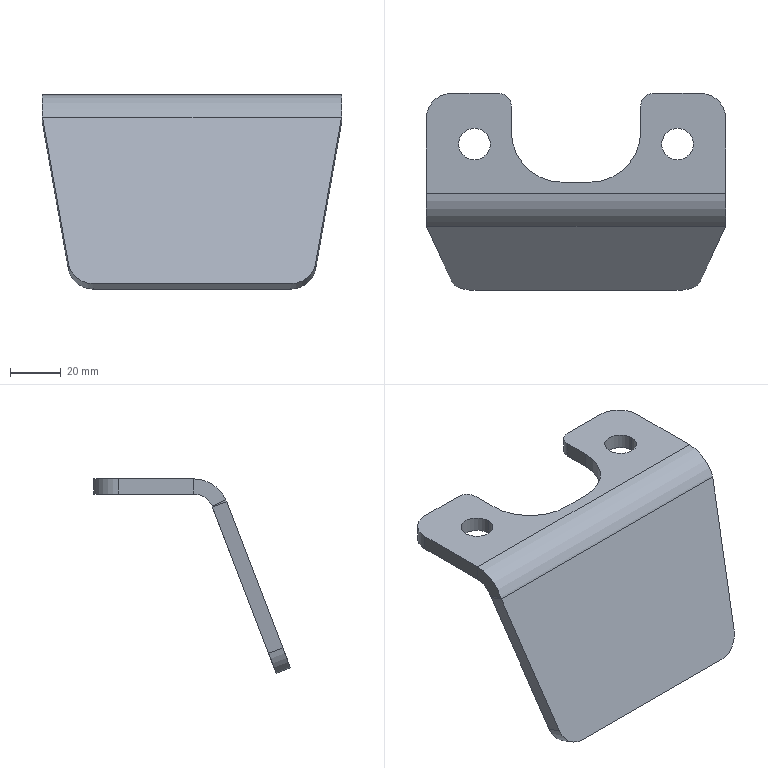Part | SolidWorks | features FlatPattern 1, SM3dBend 1, SMBaseFlange 1, SheetMetal 1, UnFold 1 | 1 solid | 32 faces | box 118 x 77.569 x 76.575 mm | volume 70276 mm3 | plane 16 | cylinder 14 | spline 2 | commonest cylinder face diameters 12.5 x4 20 x4 10 x2 40 x2 16 x1 28 x1
STEP:
#1=CARTESIAN_POINT('',(12.75,-20.,6.));
#2=VERTEX_POINT('',#1);
#3=CARTESIAN_POINT('',(25.25,-20.,6.));
#4=VERTEX_POINT('',#3);
#5=CARTESIAN_POINT('',(19.,-20.,6.));
#6=DIRECTION('',(0.,0.,1.));
#7=DIRECTION('',(1.,0.,0.));
#8=AXIS2_PLACEMENT_3D('',#5,#6,#7);
#9=CIRCLE('',#8,6.25);
#10=EDGE_CURVE('',#2,#4,#9,.T.);
#11=ORIENTED_EDGE('',*,*,#10,.T.);
#12=CARTESIAN_POINT('',(25.25,-20.,0.));
#13=VERTEX_POINT('',#12);
#14=CARTESIAN_POINT('',(25.25,-20.,6.));
#15=DIRECTION('',(0.,0.,-1.));
#16=VECTOR('',#15,1000.);
#17=LINE('',#14,#16);
#18=EDGE_CURVE('',#4,#13,#17,.T.);
#19=ORIENTED_EDGE('',*,*,#18,.T.);
#20=CARTESIAN_POINT('',(12.75,-20.,0.));
#21=VERTEX_POINT('',#20);
#22=CARTESIAN_POINT('',(19.,-20.,0.));
#23=DIRECTION('',(0.,0.,1.));
#24=DIRECTION('',(1.,0.,0.));
#25=AXIS2_PLACEMENT_3D('',#22,#23,#24);
#26=CIRCLE('',#25,6.25);
#27=EDGE_CURVE('',#21,#13,#26,.T.);
#28=ORIENTED_EDGE('',*,*,#27,.F.);
#29=CARTESIAN_POINT('',(12.75,-20.,6.));
#30=DIRECTION('',(0.,0.,-1.));
#31=VECTOR('',#30,1000.);
#32=LINE('',#29,#31);
#33=EDGE_CURVE('',#2,#21,#32,.T.);
#34=ORIENTED_EDGE('',*,*,#33,.F.);
#35=EDGE_LOOP('',(#11,#19,#28,#34));
#36=FACE_OUTER_BOUND('',#35,.T.);
#37=CARTESIAN_POINT('',(19.,-20.,6.));
#38=DIRECTION('',(0.,0.,-1.));
#39=DIRECTION('',(-1.,0.,0.));
#40=AXIS2_PLACEMENT_3D('',#37,#38,#39);
#41=CYLINDRICAL_SURFACE('',#40,6.25);
#42=ADVANCED_FACE('',(#36),#41,.F.);
#43=CARTESIAN_POINT('',(92.75,-20.,6.));
#44=VERTEX_POINT('',#43);
#45=CARTESIAN_POINT('',(105.25,-20.,6.));
#46=VERTEX_POINT('',#45);
#47=CARTESIAN_POINT('',(99.,-20.,6.));
#48=DIRECTION('',(0.,0.,1.));
#49=DIRECTION('',(1.,0.,0.));
#50=AXIS2_PLACEMENT_3D('',#47,#48,#49);
#51=CIRCLE('',#50,6.25);
#52=EDGE_CURVE('',#44,#46,#51,.T.);
#53=ORIENTED_EDGE('',*,*,#52,.T.);
#54=CARTESIAN_POINT('',(105.25,-20.,0.));
#55=VERTEX_POINT('',#54);
#56=CARTESIAN_POINT('',(105.25,-20.,6.));
#57=DIRECTION('',(0.,0.,-1.));
#58=VECTOR('',#57,1000.);
#59=LINE('',#56,#58);
#60=EDGE_CURVE('',#46,#55,#59,.T.);
#61=ORIENTED_EDGE('',*,*,#60,.T.);
#62=CARTESIAN_POINT('',(92.75,-20.,0.));
#63=VERTEX_POINT('',#62);
#64=CARTESIAN_POINT('',(99.,-20.,0.));
#65=DIRECTION('',(0.,0.,1.));
#66=DIRECTION('',(1.,0.,0.));
#67=AXIS2_PLACEMENT_3D('',#64,#65,#66);
#68=CIRCLE('',#67,6.25);
#69=EDGE_CURVE('',#63,#55,#68,.T.);
#70=ORIENTED_EDGE('',*,*,#69,.F.);
#71=CARTESIAN_POINT('',(92.75,-20.,6.));
#72=DIRECTION('',(0.,0.,-1.));
#73=VECTOR('',#72,1000.);
#74=LINE('',#71,#73);
#75=EDGE_CURVE('',#44,#63,#74,.T.);
#76=ORIENTED_EDGE('',*,*,#75,.F.);
#77=EDGE_LOOP('',(#53,#61,#70,#76));
#78=FACE_OUTER_BOUND('',#77,.T.);
#79=CARTESIAN_POINT('',(99.,-20.,6.));
#80=DIRECTION('',(0.,0.,-1.));
#81=DIRECTION('',(-1.,0.,0.));
#82=AXIS2_PLACEMENT_3D('',#79,#80,#81);
#83=CYLINDRICAL_SURFACE('',#82,6.25);
#84=ADVANCED_FACE('',(#78),#83,.F.);
#85=CARTESIAN_POINT('',(107.685,-74.57,-60.613));
#86=VERTEX_POINT('',#85);
#87=CARTESIAN_POINT('',(117.9,-52.448,-2.983));
#88=VERTEX_POINT('',#87);
#89=CARTESIAN_POINT('',(107.685,-74.57,-60.613));
#90=DIRECTION('',(0.1633,0.3536,0.9211));
#91=VECTOR('',#90,1000.);
#92=LINE('',#89,#91);
#93=EDGE_CURVE('',#86,#88,#92,.T.);
#94=ORIENTED_EDGE('',*,*,#93,.T.);
#95=CARTESIAN_POINT('',(0.09971,-52.448,-2.983));
#96=VERTEX_POINT('',#95);
#97=CARTESIAN_POINT('',(20.181,-52.448,-2.983));
#98=DIRECTION('',(-1.,0.,0.));
#99=VECTOR('',#98,1000.);
#100=LINE('',#97,#99);
#101=EDGE_CURVE('',#88,#96,#100,.T.);
#102=ORIENTED_EDGE('',*,*,#101,.T.);
#103=CARTESIAN_POINT('',(10.315,-74.57,-60.613));
#104=VERTEX_POINT('',#103);
#105=CARTESIAN_POINT('',(0.,-52.232,-2.42));
#106=DIRECTION('',(0.1633,-0.3536,-0.9211));
#107=VECTOR('',#106,1000.);
#108=LINE('',#105,#107);
#109=EDGE_CURVE('',#96,#104,#108,.T.);
#110=ORIENTED_EDGE('',*,*,#109,.T.);
#111=CARTESIAN_POINT('',(20.181,-77.569,-68.424));
#112=VERTEX_POINT('',#111);
#113=CARTESIAN_POINT('',(20.181,-73.985,-59.089));
#114=DIRECTION('',(0.,-0.9336,0.3584));
#115=DIRECTION('',(1.,0.,0.));
#116=AXIS2_PLACEMENT_3D('',#113,#114,#115);
#117=CIRCLE('',#116,10.);
#118=EDGE_CURVE('',#104,#112,#117,.T.);
#119=ORIENTED_EDGE('',*,*,#118,.T.);
#120=CARTESIAN_POINT('',(97.819,-77.569,-68.424));
#121=VERTEX_POINT('',#120);
#122=CARTESIAN_POINT('',(20.181,-77.569,-68.424));
#123=DIRECTION('',(1.,0.,0.));
#124=VECTOR('',#123,1000.);
#125=LINE('',#122,#124);
#126=EDGE_CURVE('',#112,#121,#125,.T.);
#127=ORIENTED_EDGE('',*,*,#126,.T.);
#128=CARTESIAN_POINT('',(97.819,-73.985,-59.089));
#129=DIRECTION('',(0.,-0.9336,0.3584));
#130=DIRECTION('',(1.,0.,0.));
#131=AXIS2_PLACEMENT_3D('',#128,#129,#130);
#132=CIRCLE('',#131,10.);
#133=EDGE_CURVE('',#121,#86,#132,.T.);
#134=ORIENTED_EDGE('',*,*,#133,.T.);
#135=EDGE_LOOP('',(#94,#102,#110,#119,#127,#134));
#136=FACE_OUTER_BOUND('',#135,.T.);
#137=CARTESIAN_POINT('',(20.181,-73.985,-59.089));
#138=DIRECTION('',(0.,-0.9336,0.3584));
#139=DIRECTION('',(1.,0.,0.));
#140=AXIS2_PLACEMENT_3D('',#137,#138,#139);
#141=PLANE('',#140);
#142=ADVANCED_FACE('',(#136),#141,.T.);
#143=CARTESIAN_POINT('',(117.9,-46.847,-5.133));
#144=VERTEX_POINT('',#143);
#145=CARTESIAN_POINT('',(0.09971,-46.847,-5.133));
#146=VERTEX_POINT('',#145);
#147=CARTESIAN_POINT('',(20.181,-46.847,-5.133));
#148=DIRECTION('',(-1.,0.,0.));
#149=VECTOR('',#148,1000.);
#150=LINE('',#147,#149);
#151=EDGE_CURVE('',#144,#146,#150,.T.);
#152=ORIENTED_EDGE('',*,*,#151,.F.);
#153=CARTESIAN_POINT('',(107.685,-68.969,-62.763));
#154=VERTEX_POINT('',#153);
#155=CARTESIAN_POINT('',(107.685,-68.969,-62.763));
#156=DIRECTION('',(0.1633,0.3536,0.9211));
#157=VECTOR('',#156,1000.);
#158=LINE('',#155,#157);
#159=EDGE_CURVE('',#154,#144,#158,.T.);
#160=ORIENTED_EDGE('',*,*,#159,.F.);
#161=CARTESIAN_POINT('',(97.819,-71.967,-70.575));
#162=VERTEX_POINT('',#161);
#163=CARTESIAN_POINT('',(97.819,-68.384,-61.239));
#164=DIRECTION('',(0.,-0.9336,0.3584));
#165=DIRECTION('',(1.,0.,0.));
#166=AXIS2_PLACEMENT_3D('',#163,#164,#165);
#167=CIRCLE('',#166,10.);
#168=EDGE_CURVE('',#162,#154,#167,.T.);
#169=ORIENTED_EDGE('',*,*,#168,.F.);
#170=CARTESIAN_POINT('',(20.181,-71.967,-70.575));
#171=VERTEX_POINT('',#170);
#172=CARTESIAN_POINT('',(20.181,-71.967,-70.575));
#173=DIRECTION('',(1.,0.,0.));
#174=VECTOR('',#173,1000.);
#175=LINE('',#172,#174);
#176=EDGE_CURVE('',#171,#162,#175,.T.);
#177=ORIENTED_EDGE('',*,*,#176,.F.);
#178=CARTESIAN_POINT('',(10.315,-68.969,-62.763));
#179=VERTEX_POINT('',#178);
#180=CARTESIAN_POINT('',(20.181,-68.384,-61.239));
#181=DIRECTION('',(0.,-0.9336,0.3584));
#182=DIRECTION('',(1.,0.,0.));
#183=AXIS2_PLACEMENT_3D('',#180,#181,#182);
#184=CIRCLE('',#183,10.);
#185=EDGE_CURVE('',#179,#171,#184,.T.);
#186=ORIENTED_EDGE('',*,*,#185,.F.);
#187=CARTESIAN_POINT('',(0.,-46.631,-4.571));
#188=DIRECTION('',(0.1633,-0.3536,-0.9211));
#189=VECTOR('',#188,1000.);
#190=LINE('',#187,#189);
#191=EDGE_CURVE('',#146,#179,#190,.T.);
#192=ORIENTED_EDGE('',*,*,#191,.F.);
#193=EDGE_LOOP('',(#152,#160,#169,#177,#186,#192));
#194=FACE_OUTER_BOUND('',#193,.T.);
#195=CARTESIAN_POINT('',(20.181,-68.384,-61.239));
#196=DIRECTION('',(0.,-0.9336,0.3584));
#197=DIRECTION('',(1.,0.,0.));
#198=AXIS2_PLACEMENT_3D('',#195,#196,#197);
#199=PLANE('',#198);
#200=ADVANCED_FACE('',(#194),#199,.F.);
#201=CARTESIAN_POINT('',(0.09971,-46.847,-5.133));
#202=CARTESIAN_POINT('',(0.09971,-52.448,-2.983));
#203=B_SPLINE_CURVE_WITH_KNOTS('',1,(#201,#202),.UNSPECIFIED.,.F.,.F.,(2,2),(0.,1.),.UNSPECIFIED.);
#204=EDGE_CURVE('',#146,#96,#203,.T.);
#205=ORIENTED_EDGE('',*,*,#204,.F.);
#206=ORIENTED_EDGE('',*,*,#191,.T.);
#207=CARTESIAN_POINT('',(10.315,-74.57,-60.613));
#208=DIRECTION('',(0.,0.9336,-0.3584));
#209=VECTOR('',#208,1000.);
#210=LINE('',#207,#209);
#211=EDGE_CURVE('',#104,#179,#210,.T.);
#212=ORIENTED_EDGE('',*,*,#211,.F.);
#213=ORIENTED_EDGE('',*,*,#109,.F.);
#214=EDGE_LOOP('',(#205,#206,#212,#213));
#215=FACE_OUTER_BOUND('',#214,.T.);
#216=CARTESIAN_POINT('',(0.,-52.232,-2.42));
#217=DIRECTION('',(0.9866,0.05851,0.1524));
#218=DIRECTION('',(-0.1633,0.3536,0.9211));
#219=AXIS2_PLACEMENT_3D('',#216,#217,#218);
#220=PLANE('',#219);
#221=ADVANCED_FACE('',(#215),#220,.F.);
#222=ORIENTED_EDGE('',*,*,#185,.T.);
#223=CARTESIAN_POINT('',(20.181,-77.569,-68.424));
#224=DIRECTION('',(0.,0.9336,-0.3584));
#225=VECTOR('',#224,1000.);
#226=LINE('',#223,#225);
#227=EDGE_CURVE('',#112,#171,#226,.T.);
#228=ORIENTED_EDGE('',*,*,#227,.F.);
#229=ORIENTED_EDGE('',*,*,#118,.F.);
#230=ORIENTED_EDGE('',*,*,#211,.T.);
#231=EDGE_LOOP('',(#222,#228,#229,#230));
#232=FACE_OUTER_BOUND('',#231,.T.);
#233=CARTESIAN_POINT('',(20.181,-73.985,-59.089));
#234=DIRECTION('',(0.,0.9336,-0.3584));
#235=DIRECTION('',(-1.,0.,0.));
#236=AXIS2_PLACEMENT_3D('',#233,#234,#235);
#237=CYLINDRICAL_SURFACE('',#236,10.);
#238=ADVANCED_FACE('',(#232),#237,.T.);
#239=ORIENTED_EDGE('',*,*,#176,.T.);
#240=CARTESIAN_POINT('',(97.819,-77.569,-68.424));
#241=DIRECTION('',(0.,0.9336,-0.3584));
#242=VECTOR('',#241,1000.);
#243=LINE('',#240,#242);
#244=EDGE_CURVE('',#121,#162,#243,.T.);
#245=ORIENTED_EDGE('',*,*,#244,.F.);
#246=ORIENTED_EDGE('',*,*,#126,.F.);
#247=ORIENTED_EDGE('',*,*,#227,.T.);
#248=EDGE_LOOP('',(#239,#245,#246,#247));
#249=FACE_OUTER_BOUND('',#248,.T.);
#250=CARTESIAN_POINT('',(20.181,-77.569,-68.424));
#251=DIRECTION('',(0.,0.3584,0.9336));
#252=DIRECTION('',(-1.,0.,0.));
#253=AXIS2_PLACEMENT_3D('',#250,#251,#252);
#254=PLANE('',#253);
#255=ADVANCED_FACE('',(#249),#254,.F.);
#256=ORIENTED_EDGE('',*,*,#168,.T.);
#257=CARTESIAN_POINT('',(107.685,-74.57,-60.613));
#258=DIRECTION('',(0.,0.9336,-0.3584));
#259=VECTOR('',#258,1000.);
#260=LINE('',#257,#259);
#261=EDGE_CURVE('',#86,#154,#260,.T.);
#262=ORIENTED_EDGE('',*,*,#261,.F.);
#263=ORIENTED_EDGE('',*,*,#133,.F.);
#264=ORIENTED_EDGE('',*,*,#244,.T.);
#265=EDGE_LOOP('',(#256,#262,#263,#264));
#266=FACE_OUTER_BOUND('',#265,.T.);
#267=CARTESIAN_POINT('',(97.819,-73.985,-59.089));
#268=DIRECTION('',(0.,0.9336,-0.3584));
#269=DIRECTION('',(-1.,0.,0.));
#270=AXIS2_PLACEMENT_3D('',#267,#268,#269);
#271=CYLINDRICAL_SURFACE('',#270,10.);
#272=ADVANCED_FACE('',(#266),#271,.T.);
#273=CARTESIAN_POINT('',(117.9,-52.448,-2.983));
#274=CARTESIAN_POINT('',(117.9,-46.847,-5.133));
#275=B_SPLINE_CURVE_WITH_KNOTS('',1,(#273,#274),.UNSPECIFIED.,.F.,.F.,(2,2),(0.,1.),.UNSPECIFIED.);
#276=EDGE_CURVE('',#88,#144,#275,.T.);
#277=ORIENTED_EDGE('',*,*,#276,.F.);
#278=ORIENTED_EDGE('',*,*,#93,.F.);
#279=ORIENTED_EDGE('',*,*,#261,.T.);
#280=ORIENTED_EDGE('',*,*,#159,.T.);
#281=EDGE_LOOP('',(#277,#278,#279,#280));
#282=FACE_OUTER_BOUND('',#281,.T.);
#283=CARTESIAN_POINT('',(107.685,-74.57,-60.613));
#284=DIRECTION('',(-0.9866,0.05851,0.1524));
#285=DIRECTION('',(-0.1633,-0.3536,-0.9211));
#286=AXIS2_PLACEMENT_3D('',#283,#284,#285);
#287=PLANE('',#286);
#288=ADVANCED_FACE('',(#282),#287,.F.);
#289=ORIENTED_EDGE('',*,*,#60,.F.);
#290=CARTESIAN_POINT('',(99.,-20.,6.));
#291=DIRECTION('',(0.,0.,1.));
#292=DIRECTION('',(1.,0.,0.));
#293=AXIS2_PLACEMENT_3D('',#290,#291,#292);
#294=CIRCLE('',#293,6.25);
#295=EDGE_CURVE('',#46,#44,#294,.T.);
#296=ORIENTED_EDGE('',*,*,#295,.T.);
#297=ORIENTED_EDGE('',*,*,#75,.T.);
#298=CARTESIAN_POINT('',(99.,-20.,0.));
#299=DIRECTION('',(0.,0.,1.));
#300=DIRECTION('',(1.,0.,0.));
#301=AXIS2_PLACEMENT_3D('',#298,#299,#300);
#302=CIRCLE('',#301,6.25);
#303=EDGE_CURVE('',#55,#63,#302,.T.);
#304=ORIENTED_EDGE('',*,*,#303,.F.);
#305=EDGE_LOOP('',(#289,#296,#297,#304));
#306=FACE_OUTER_BOUND('',#305,.T.);
#307=CARTESIAN_POINT('',(99.,-20.,6.));
#308=DIRECTION('',(0.,0.,-1.));
#309=DIRECTION('',(-1.,0.,0.));
#310=AXIS2_PLACEMENT_3D('',#307,#308,#309);
#311=CYLINDRICAL_SURFACE('',#310,6.25);
#312=ADVANCED_FACE('',(#306),#311,.F.);
#313=ORIENTED_EDGE('',*,*,#18,.F.);
#314=CARTESIAN_POINT('',(19.,-20.,6.));
#315=DIRECTION('',(0.,0.,1.));
#316=DIRECTION('',(1.,0.,0.));
#317=AXIS2_PLACEMENT_3D('',#314,#315,#316);
#318=CIRCLE('',#317,6.25);
#319=EDGE_CURVE('',#4,#2,#318,.T.);
#320=ORIENTED_EDGE('',*,*,#319,.T.);
#321=ORIENTED_EDGE('',*,*,#33,.T.);
#322=CARTESIAN_POINT('',(19.,-20.,0.));
#323=DIRECTION('',(0.,0.,1.));
#324=DIRECTION('',(1.,0.,0.));
#325=AXIS2_PLACEMENT_3D('',#322,#323,#324);
#326=CIRCLE('',#325,6.25);
#327=EDGE_CURVE('',#13,#21,#326,.T.);
#328=ORIENTED_EDGE('',*,*,#327,.F.);
#329=EDGE_LOOP('',(#313,#320,#321,#328));
#330=FACE_OUTER_BOUND('',#329,.T.);
#331=CARTESIAN_POINT('',(19.,-20.,6.));
#332=DIRECTION('',(0.,0.,-1.));
#333=DIRECTION('',(-1.,0.,0.));
#334=AXIS2_PLACEMENT_3D('',#331,#332,#333);
#335=CYLINDRICAL_SURFACE('',#334,6.25);
#336=ADVANCED_FACE('',(#330),#335,.F.);
#337=CARTESIAN_POINT('',(10.,0.,0.));
#338=VERTEX_POINT('',#337);
#339=CARTESIAN_POINT('',(0.,-10.,0.));
#340=VERTEX_POINT('',#339);
#341=CARTESIAN_POINT('',(10.,-10.,0.));
#342=DIRECTION('',(0.,0.,1.));
#343=DIRECTION('',(-1.,0.,0.));
#344=AXIS2_PLACEMENT_3D('',#341,#342,#343);
#345=CIRCLE('',#344,10.);
#346=EDGE_CURVE('',#338,#340,#345,.T.);
#347=ORIENTED_EDGE('',*,*,#346,.T.);
#348=CARTESIAN_POINT('',(0.,-10.,6.));
#349=VERTEX_POINT('',#348);
#350=CARTESIAN_POINT('',(0.,-10.,6.));
#351=DIRECTION('',(0.,0.,-1.));
#352=VECTOR('',#351,1000.);
#353=LINE('',#350,#352);
#354=EDGE_CURVE('',#349,#340,#353,.T.);
#355=ORIENTED_EDGE('',*,*,#354,.F.);
#356=CARTESIAN_POINT('',(10.,0.,6.));
#357=VERTEX_POINT('',#356);
#358=CARTESIAN_POINT('',(10.,-10.,6.));
#359=DIRECTION('',(0.,0.,1.));
#360=DIRECTION('',(-1.,0.,0.));
#361=AXIS2_PLACEMENT_3D('',#358,#359,#360);
#362=CIRCLE('',#361,10.);
#363=EDGE_CURVE('',#357,#349,#362,.T.);
#364=ORIENTED_EDGE('',*,*,#363,.F.);
#365=CARTESIAN_POINT('',(10.,0.,6.));
#366=DIRECTION('',(0.,0.,-1.));
#367=VECTOR('',#366,1000.);
#368=LINE('',#365,#367);
#369=EDGE_CURVE('',#357,#338,#368,.T.);
#370=ORIENTED_EDGE('',*,*,#369,.T.);
#371=EDGE_LOOP('',(#347,#355,#364,#370));
#372=FACE_OUTER_BOUND('',#371,.T.);
#373=CARTESIAN_POINT('',(10.,-10.,6.));
#374=DIRECTION('',(0.,0.,-1.));
#375=DIRECTION('',(-1.,0.,0.));
#376=AXIS2_PLACEMENT_3D('',#373,#374,#375);
#377=CYLINDRICAL_SURFACE('',#376,10.);
#378=ADVANCED_FACE('',(#372),#377,.T.);
#379=CARTESIAN_POINT('',(28.5,0.,0.));
#380=VERTEX_POINT('',#379);
#381=CARTESIAN_POINT('',(28.5,0.,0.));
#382=DIRECTION('',(-1.,0.,0.));
#383=VECTOR('',#382,1000.);
#384=LINE('',#381,#383);
#385=EDGE_CURVE('',#380,#338,#384,.T.);
#386=ORIENTED_EDGE('',*,*,#385,.T.);
#387=ORIENTED_EDGE('',*,*,#369,.F.);
#388=CARTESIAN_POINT('',(28.5,0.,6.));
#389=VERTEX_POINT('',#388);
#390=CARTESIAN_POINT('',(28.5,0.,6.));
#391=DIRECTION('',(-1.,0.,0.));
#392=VECTOR('',#391,1000.);
#393=LINE('',#390,#392);
#394=EDGE_CURVE('',#389,#357,#393,.T.);
#395=ORIENTED_EDGE('',*,*,#394,.F.);
#396=CARTESIAN_POINT('',(28.5,0.,6.));
#397=DIRECTION('',(0.,0.,-1.));
#398=VECTOR('',#397,1000.);
#399=LINE('',#396,#398);
#400=EDGE_CURVE('',#389,#380,#399,.T.);
#401=ORIENTED_EDGE('',*,*,#400,.T.);
#402=EDGE_LOOP('',(#386,#387,#395,#401));
#403=FACE_OUTER_BOUND('',#402,.T.);
#404=CARTESIAN_POINT('',(28.5,0.,6.));
#405=DIRECTION('',(0.,-1.,0.));
#406=DIRECTION('',(1.,0.,0.));
#407=AXIS2_PLACEMENT_3D('',#404,#405,#406);
#408=PLANE('',#407);
#409=ADVANCED_FACE('',(#403),#408,.F.);
#410=CARTESIAN_POINT('',(33.5,-5.,0.));
#411=VERTEX_POINT('',#410);
#412=CARTESIAN_POINT('',(28.5,-5.,0.));
#413=DIRECTION('',(0.,0.,1.));
#414=DIRECTION('',(1.,0.,0.));
#415=AXIS2_PLACEMENT_3D('',#412,#413,#414);
#416=CIRCLE('',#415,5.);
#417=EDGE_CURVE('',#411,#380,#416,.T.);
#418=ORIENTED_EDGE('',*,*,#417,.T.);
#419=ORIENTED_EDGE('',*,*,#400,.F.);
#420=CARTESIAN_POINT('',(33.5,-5.,6.));
#421=VERTEX_POINT('',#420);
#422=CARTESIAN_POINT('',(28.5,-5.,6.));
#423=DIRECTION('',(0.,0.,1.));
#424=DIRECTION('',(1.,0.,0.));
#425=AXIS2_PLACEMENT_3D('',#422,#423,#424);
#426=CIRCLE('',#425,5.);
#427=EDGE_CURVE('',#421,#389,#426,.T.);
#428=ORIENTED_EDGE('',*,*,#427,.F.);
#429=CARTESIAN_POINT('',(33.5,-5.,6.));
#430=DIRECTION('',(0.,0.,-1.));
#431=VECTOR('',#430,1000.);
#432=LINE('',#429,#431);
#433=EDGE_CURVE('',#421,#411,#432,.T.);
#434=ORIENTED_EDGE('',*,*,#433,.T.);
#435=EDGE_LOOP('',(#418,#419,#428,#434));
#436=FACE_OUTER_BOUND('',#435,.T.);
#437=CARTESIAN_POINT('',(28.5,-5.,6.));
#438=DIRECTION('',(0.,0.,-1.));
#439=DIRECTION('',(-1.,0.,0.));
#440=AXIS2_PLACEMENT_3D('',#437,#438,#439);
#441=CYLINDRICAL_SURFACE('',#440,5.);
#442=ADVANCED_FACE('',(#436),#441,.T.);
#443=CARTESIAN_POINT('',(33.5,-15.,0.));
#444=VERTEX_POINT('',#443);
#445=CARTESIAN_POINT('',(33.5,-15.,0.));
#446=DIRECTION('',(0.,1.,0.));
#447=VECTOR('',#446,1000.);
#448=LINE('',#445,#447);
#449=EDGE_CURVE('',#444,#411,#448,.T.);
#450=ORIENTED_EDGE('',*,*,#449,.T.);
#451=ORIENTED_EDGE('',*,*,#433,.F.);
#452=CARTESIAN_POINT('',(33.5,-15.,6.));
#453=VERTEX_POINT('',#452);
#454=CARTESIAN_POINT('',(33.5,-15.,6.));
#455=DIRECTION('',(0.,1.,0.));
#456=VECTOR('',#455,1000.);
#457=LINE('',#454,#456);
#458=EDGE_CURVE('',#453,#421,#457,.T.);
#459=ORIENTED_EDGE('',*,*,#458,.F.);
#460=CARTESIAN_POINT('',(33.5,-15.,6.));
#461=DIRECTION('',(0.,0.,-1.));
#462=VECTOR('',#461,1000.);
#463=LINE('',#460,#462);
#464=EDGE_CURVE('',#453,#444,#463,.T.);
#465=ORIENTED_EDGE('',*,*,#464,.T.);
#466=EDGE_LOOP('',(#450,#451,#459,#465));
#467=FACE_OUTER_BOUND('',#466,.T.);
#468=CARTESIAN_POINT('',(33.5,-15.,6.));
#469=DIRECTION('',(-1.,0.,0.));
#470=DIRECTION('',(0.,0.,1.));
#471=AXIS2_PLACEMENT_3D('',#468,#469,#470);
#472=PLANE('',#471);
#473=ADVANCED_FACE('',(#467),#472,.F.);
#474=CARTESIAN_POINT('',(53.5,-35.,0.));
#475=VERTEX_POINT('',#474);
#476=CARTESIAN_POINT('',(53.5,-15.,0.));
#477=DIRECTION('',(0.,0.,-1.));
#478=DIRECTION('',(-1.,0.,0.));
#479=AXIS2_PLACEMENT_3D('',#476,#477,#478);
#480=CIRCLE('',#479,20.);
#481=EDGE_CURVE('',#475,#444,#480,.T.);
#482=ORIENTED_EDGE('',*,*,#481,.T.);
#483=ORIENTED_EDGE('',*,*,#464,.F.);
#484=CARTESIAN_POINT('',(53.5,-35.,6.));
#485=VERTEX_POINT('',#484);
#486=CARTESIAN_POINT('',(53.5,-15.,6.));
#487=DIRECTION('',(0.,0.,-1.));
#488=DIRECTION('',(-1.,0.,0.));
#489=AXIS2_PLACEMENT_3D('',#486,#487,#488);
#490=CIRCLE('',#489,20.);
#491=EDGE_CURVE('',#485,#453,#490,.T.);
#492=ORIENTED_EDGE('',*,*,#491,.F.);
#493=CARTESIAN_POINT('',(53.5,-35.,6.));
#494=DIRECTION('',(0.,0.,-1.));
#495=VECTOR('',#494,1000.);
#496=LINE('',#493,#495);
#497=EDGE_CURVE('',#485,#475,#496,.T.);
#498=ORIENTED_EDGE('',*,*,#497,.T.);
#499=EDGE_LOOP('',(#482,#483,#492,#498));
#500=FACE_OUTER_BOUND('',#499,.T.);
#501=CARTESIAN_POINT('',(53.5,-15.,6.));
#502=DIRECTION('',(0.,0.,-1.));
#503=DIRECTION('',(-1.,0.,0.));
#504=AXIS2_PLACEMENT_3D('',#501,#502,#503);
#505=CYLINDRICAL_SURFACE('',#504,20.);
#506=ADVANCED_FACE('',(#500),#505,.F.);
#507=CARTESIAN_POINT('',(64.5,-35.,0.));
#508=VERTEX_POINT('',#507);
#509=CARTESIAN_POINT('',(64.5,-35.,0.));
#510=DIRECTION('',(-1.,0.,0.));
#511=VECTOR('',#510,1000.);
#512=LINE('',#509,#511);
#513=EDGE_CURVE('',#508,#475,#512,.T.);
#514=ORIENTED_EDGE('',*,*,#513,.T.);
#515=ORIENTED_EDGE('',*,*,#497,.F.);
#516=CARTESIAN_POINT('',(64.5,-35.,6.));
#517=VERTEX_POINT('',#516);
#518=CARTESIAN_POINT('',(64.5,-35.,6.));
#519=DIRECTION('',(-1.,0.,0.));
#520=VECTOR('',#519,1000.);
#521=LINE('',#518,#520);
#522=EDGE_CURVE('',#517,#485,#521,.T.);
#523=ORIENTED_EDGE('',*,*,#522,.F.);
#524=CARTESIAN_POINT('',(64.5,-35.,6.));
#525=DIRECTION('',(0.,0.,-1.));
#526=VECTOR('',#525,1000.);
#527=LINE('',#524,#526);
#528=EDGE_CURVE('',#517,#508,#527,.T.);
#529=ORIENTED_EDGE('',*,*,#528,.T.);
#530=EDGE_LOOP('',(#514,#515,#523,#529));
#531=FACE_OUTER_BOUND('',#530,.T.);
#532=CARTESIAN_POINT('',(64.5,-35.,6.));
#533=DIRECTION('',(0.,-1.,0.));
#534=DIRECTION('',(0.,0.,-1.));
#535=AXIS2_PLACEMENT_3D('',#532,#533,#534);
#536=PLANE('',#535);
#537=ADVANCED_FACE('',(#531),#536,.F.);
#538=CARTESIAN_POINT('',(84.5,-15.,0.));
#539=VERTEX_POINT('',#538);
#540=CARTESIAN_POINT('',(64.5,-15.,0.));
#541=DIRECTION('',(0.,0.,-1.));
#542=DIRECTION('',(-1.,0.,0.));
#543=AXIS2_PLACEMENT_3D('',#540,#541,#542);
#544=CIRCLE('',#543,20.);
#545=EDGE_CURVE('',#539,#508,#544,.T.);
#546=ORIENTED_EDGE('',*,*,#545,.T.);
#547=ORIENTED_EDGE('',*,*,#528,.F.);
#548=CARTESIAN_POINT('',(84.5,-15.,6.));
#549=VERTEX_POINT('',#548);
#550=CARTESIAN_POINT('',(64.5,-15.,6.));
#551=DIRECTION('',(0.,0.,-1.));
#552=DIRECTION('',(-1.,0.,0.));
#553=AXIS2_PLACEMENT_3D('',#550,#551,#552);
#554=CIRCLE('',#553,20.);
#555=EDGE_CURVE('',#549,#517,#554,.T.);
#556=ORIENTED_EDGE('',*,*,#555,.F.);
#557=CARTESIAN_POINT('',(84.5,-15.,6.));
#558=DIRECTION('',(0.,0.,-1.));
#559=VECTOR('',#558,1000.);
#560=LINE('',#557,#559);
#561=EDGE_CURVE('',#549,#539,#560,.T.);
#562=ORIENTED_EDGE('',*,*,#561,.T.);
#563=EDGE_LOOP('',(#546,#547,#556,#562));
#564=FACE_OUTER_BOUND('',#563,.T.);
#565=CARTESIAN_POINT('',(64.5,-15.,6.));
#566=DIRECTION('',(0.,0.,-1.));
#567=DIRECTION('',(-1.,0.,0.));
#568=AXIS2_PLACEMENT_3D('',#565,#566,#567);
#569=CYLINDRICAL_SURFACE('',#568,20.);
#570=ADVANCED_FACE('',(#564),#569,.F.);
#571=CARTESIAN_POINT('',(84.5,-5.,0.));
#572=VERTEX_POINT('',#571);
#573=CARTESIAN_POINT('',(84.5,-5.,0.));
#574=DIRECTION('',(0.,-1.,0.));
#575=VECTOR('',#574,1000.);
#576=LINE('',#573,#575);
#577=EDGE_CURVE('',#572,#539,#576,.T.);
#578=ORIENTED_EDGE('',*,*,#577,.T.);
#579=ORIENTED_EDGE('',*,*,#561,.F.);
#580=CARTESIAN_POINT('',(84.5,-5.,6.));
#581=VERTEX_POINT('',#580);
#582=CARTESIAN_POINT('',(84.5,-5.,6.));
#583=DIRECTION('',(0.,-1.,0.));
#584=VECTOR('',#583,1000.);
#585=LINE('',#582,#584);
#586=EDGE_CURVE('',#581,#549,#585,.T.);
#587=ORIENTED_EDGE('',*,*,#586,.F.);
#588=CARTESIAN_POINT('',(84.5,-5.,6.));
#589=DIRECTION('',(0.,0.,-1.));
#590=VECTOR('',#589,1000.);
#591=LINE('',#588,#590);
#592=EDGE_CURVE('',#581,#572,#591,.T.);
#593=ORIENTED_EDGE('',*,*,#592,.T.);
#594=EDGE_LOOP('',(#578,#579,#587,#593));
#595=FACE_OUTER_BOUND('',#594,.T.);
#596=CARTESIAN_POINT('',(84.5,-5.,6.));
#597=DIRECTION('',(1.,0.,0.));
#598=DIRECTION('',(0.,0.,-1.));
#599=AXIS2_PLACEMENT_3D('',#596,#597,#598);
#600=PLANE('',#599);
#601=ADVANCED_FACE('',(#595),#600,.F.);
#602=CARTESIAN_POINT('',(89.5,0.,0.));
#603=VERTEX_POINT('',#602);
#604=CARTESIAN_POINT('',(89.5,-5.,0.));
#605=DIRECTION('',(0.,0.,1.));
#606=DIRECTION('',(1.,0.,0.));
#607=AXIS2_PLACEMENT_3D('',#604,#605,#606);
#608=CIRCLE('',#607,5.);
#609=EDGE_CURVE('',#603,#572,#608,.T.);
#610=ORIENTED_EDGE('',*,*,#609,.T.);
#611=ORIENTED_EDGE('',*,*,#592,.F.);
#612=CARTESIAN_POINT('',(89.5,0.,6.));
#613=VERTEX_POINT('',#612);
#614=CARTESIAN_POINT('',(89.5,-5.,6.));
#615=DIRECTION('',(0.,0.,1.));
#616=DIRECTION('',(1.,0.,0.));
#617=AXIS2_PLACEMENT_3D('',#614,#615,#616);
#618=CIRCLE('',#617,5.);
#619=EDGE_CURVE('',#613,#581,#618,.T.);
#620=ORIENTED_EDGE('',*,*,#619,.F.);
#621=CARTESIAN_POINT('',(89.5,0.,6.));
#622=DIRECTION('',(0.,0.,-1.));
#623=VECTOR('',#622,1000.);
#624=LINE('',#621,#623);
#625=EDGE_CURVE('',#613,#603,#624,.T.);
#626=ORIENTED_EDGE('',*,*,#625,.T.);
#627=EDGE_LOOP('',(#610,#611,#620,#626));
#628=FACE_OUTER_BOUND('',#627,.T.);
#629=CARTESIAN_POINT('',(89.5,-5.,6.));
#630=DIRECTION('',(0.,0.,-1.));
#631=DIRECTION('',(-1.,0.,0.));
#632=AXIS2_PLACEMENT_3D('',#629,#630,#631);
#633=CYLINDRICAL_SURFACE('',#632,5.);
#634=ADVANCED_FACE('',(#628),#633,.T.);
#635=CARTESIAN_POINT('',(108.,0.,0.));
#636=VERTEX_POINT('',#635);
#637=CARTESIAN_POINT('',(108.,0.,0.));
#638=DIRECTION('',(-1.,0.,0.));
#639=VECTOR('',#638,1000.);
#640=LINE('',#637,#639);
#641=EDGE_CURVE('',#636,#603,#640,.T.);
#642=ORIENTED_EDGE('',*,*,#641,.T.);
#643=ORIENTED_EDGE('',*,*,#625,.F.);
#644=CARTESIAN_POINT('',(108.,0.,6.));
#645=VERTEX_POINT('',#644);
#646=CARTESIAN_POINT('',(108.,0.,6.));
#647=DIRECTION('',(-1.,0.,0.));
#648=VECTOR('',#647,1000.);
#649=LINE('',#646,#648);
#650=EDGE_CURVE('',#645,#613,#649,.T.);
#651=ORIENTED_EDGE('',*,*,#650,.F.);
#652=CARTESIAN_POINT('',(108.,0.,6.));
#653=DIRECTION('',(0.,0.,-1.));
#654=VECTOR('',#653,1000.);
#655=LINE('',#652,#654);
#656=EDGE_CURVE('',#645,#636,#655,.T.);
#657=ORIENTED_EDGE('',*,*,#656,.T.);
#658=EDGE_LOOP('',(#642,#643,#651,#657));
#659=FACE_OUTER_BOUND('',#658,.T.);
#660=CARTESIAN_POINT('',(108.,0.,6.));
#661=DIRECTION('',(0.,-1.,0.));
#662=DIRECTION('',(1.,0.,0.));
#663=AXIS2_PLACEMENT_3D('',#660,#661,#662);
#664=PLANE('',#663);
#665=ADVANCED_FACE('',(#659),#664,.F.);
#666=CARTESIAN_POINT('',(118.,-10.,0.));
#667=VERTEX_POINT('',#666);
#668=CARTESIAN_POINT('',(108.,-10.,0.));
#669=DIRECTION('',(0.,0.,1.));
#670=DIRECTION('',(1.,0.,0.));
#671=AXIS2_PLACEMENT_3D('',#668,#669,#670);
#672=CIRCLE('',#671,10.);
#673=EDGE_CURVE('',#667,#636,#672,.T.);
#674=ORIENTED_EDGE('',*,*,#673,.T.);
#675=ORIENTED_EDGE('',*,*,#656,.F.);
#676=CARTESIAN_POINT('',(118.,-10.,6.));
#677=VERTEX_POINT('',#676);
#678=CARTESIAN_POINT('',(108.,-10.,6.));
#679=DIRECTION('',(0.,0.,1.));
#680=DIRECTION('',(1.,0.,0.));
#681=AXIS2_PLACEMENT_3D('',#678,#679,#680);
#682=CIRCLE('',#681,10.);
#683=EDGE_CURVE('',#677,#645,#682,.T.);
#684=ORIENTED_EDGE('',*,*,#683,.F.);
#685=CARTESIAN_POINT('',(118.,-10.,6.));
#686=DIRECTION('',(0.,0.,-1.));
#687=VECTOR('',#686,1000.);
#688=LINE('',#685,#687);
#689=EDGE_CURVE('',#677,#667,#688,.T.);
#690=ORIENTED_EDGE('',*,*,#689,.T.);
#691=EDGE_LOOP('',(#674,#675,#684,#690));
#692=FACE_OUTER_BOUND('',#691,.T.);
#693=CARTESIAN_POINT('',(108.,-10.,6.));
#694=DIRECTION('',(0.,0.,-1.));
#695=DIRECTION('',(-1.,0.,0.));
#696=AXIS2_PLACEMENT_3D('',#693,#694,#695);
#697=CYLINDRICAL_SURFACE('',#696,10.);
#698=ADVANCED_FACE('',(#692),#697,.T.);
#699=CARTESIAN_POINT('',(118.,-39.378,6.));
#700=VERTEX_POINT('',#699);
#701=CARTESIAN_POINT('',(0.,-39.378,6.));
#702=VERTEX_POINT('',#701);
#703=CARTESIAN_POINT('',(20.181,-39.378,6.));
#704=DIRECTION('',(-1.,0.,0.));
#705=VECTOR('',#704,1000.);
#706=LINE('',#703,#705);
#707=EDGE_CURVE('',#700,#702,#706,.T.);
#708=ORIENTED_EDGE('',*,*,#707,.F.);
#709=CARTESIAN_POINT('',(118.,-51.3,6.));
#710=DIRECTION('',(0.,1.,0.));
#711=VECTOR('',#710,1000.);
#712=LINE('',#709,#711);
#713=EDGE_CURVE('',#700,#677,#712,.T.);
#714=ORIENTED_EDGE('',*,*,#713,.T.);
#715=ORIENTED_EDGE('',*,*,#683,.T.);
#716=ORIENTED_EDGE('',*,*,#650,.T.);
#717=ORIENTED_EDGE('',*,*,#619,.T.);
#718=ORIENTED_EDGE('',*,*,#586,.T.);
#719=ORIENTED_EDGE('',*,*,#555,.T.);
#720=ORIENTED_EDGE('',*,*,#522,.T.);
#721=ORIENTED_EDGE('',*,*,#491,.T.);
#722=ORIENTED_EDGE('',*,*,#458,.T.);
#723=ORIENTED_EDGE('',*,*,#427,.T.);
#724=ORIENTED_EDGE('',*,*,#394,.T.);
#725=ORIENTED_EDGE('',*,*,#363,.T.);
#726=CARTESIAN_POINT('',(0.,-10.,6.));
#727=DIRECTION('',(0.,-1.,0.));
#728=VECTOR('',#727,1000.);
#729=LINE('',#726,#728);
#730=EDGE_CURVE('',#349,#702,#729,.T.);
#731=ORIENTED_EDGE('',*,*,#730,.T.);
#732=EDGE_LOOP('',(#708,#714,#715,#716,#717,#718,#719,#720,#721,#722,#723,#724,#725,#731));
#733=FACE_OUTER_BOUND('',#732,.T.);
#734=ORIENTED_EDGE('',*,*,#10,.F.);
#735=ORIENTED_EDGE('',*,*,#319,.F.);
#736=EDGE_LOOP('',(#734,#735));
#737=FACE_BOUND('',#736,.T.);
#738=ORIENTED_EDGE('',*,*,#52,.F.);
#739=ORIENTED_EDGE('',*,*,#295,.F.);
#740=EDGE_LOOP('',(#738,#739));
#741=FACE_BOUND('',#740,.T.);
#742=CARTESIAN_POINT('',(20.181,-112.,6.));
#743=DIRECTION('',(0.,0.,1.));
#744=DIRECTION('',(1.,0.,0.));
#745=AXIS2_PLACEMENT_3D('',#742,#743,#744);
#746=PLANE('',#745);
#747=ADVANCED_FACE('',(#733,#737,#741),#746,.T.);
#748=ORIENTED_EDGE('',*,*,#713,.F.);
#749=CARTESIAN_POINT('',(118.,-39.378,0.));
#750=VERTEX_POINT('',#749);
#751=CARTESIAN_POINT('',(118.,-39.378,6.));
#752=DIRECTION('',(0.,0.,-1.));
#753=VECTOR('',#752,1000.);
#754=LINE('',#751,#753);
#755=EDGE_CURVE('',#700,#750,#754,.T.);
#756=ORIENTED_EDGE('',*,*,#755,.T.);
#757=CARTESIAN_POINT('',(118.,-51.3,0.));
#758=DIRECTION('',(0.,1.,0.));
#759=VECTOR('',#758,1000.);
#760=LINE('',#757,#759);
#761=EDGE_CURVE('',#750,#667,#760,.T.);
#762=ORIENTED_EDGE('',*,*,#761,.T.);
#763=ORIENTED_EDGE('',*,*,#689,.F.);
#764=EDGE_LOOP('',(#748,#756,#762,#763));
#765=FACE_OUTER_BOUND('',#764,.T.);
#766=CARTESIAN_POINT('',(118.,-51.3,6.));
#767=DIRECTION('',(-1.,0.,0.));
#768=DIRECTION('',(0.,-1.,0.));
#769=AXIS2_PLACEMENT_3D('',#766,#767,#768);
#770=PLANE('',#769);
#771=ADVANCED_FACE('',(#765),#770,.F.);
#772=ORIENTED_EDGE('',*,*,#27,.T.);
#773=ORIENTED_EDGE('',*,*,#327,.T.);
#774=EDGE_LOOP('',(#772,#773));
#775=FACE_BOUND('',#774,.T.);
#776=ORIENTED_EDGE('',*,*,#69,.T.);
#777=ORIENTED_EDGE('',*,*,#303,.T.);
#778=EDGE_LOOP('',(#776,#777));
#779=FACE_BOUND('',#778,.T.);
#780=ORIENTED_EDGE('',*,*,#761,.F.);
#781=CARTESIAN_POINT('',(0.,-39.378,0.));
#782=VERTEX_POINT('',#781);
#783=CARTESIAN_POINT('',(20.181,-39.378,0.));
#784=DIRECTION('',(-1.,0.,0.));
#785=VECTOR('',#784,1000.);
#786=LINE('',#783,#785);
#787=EDGE_CURVE('',#750,#782,#786,.T.);
#788=ORIENTED_EDGE('',*,*,#787,.T.);
#789=CARTESIAN_POINT('',(0.,-10.,0.));
#790=DIRECTION('',(0.,-1.,0.));
#791=VECTOR('',#790,1000.);
#792=LINE('',#789,#791);
#793=EDGE_CURVE('',#340,#782,#792,.T.);
#794=ORIENTED_EDGE('',*,*,#793,.F.);
#795=ORIENTED_EDGE('',*,*,#346,.F.);
#796=ORIENTED_EDGE('',*,*,#385,.F.);
#797=ORIENTED_EDGE('',*,*,#417,.F.);
#798=ORIENTED_EDGE('',*,*,#449,.F.);
#799=ORIENTED_EDGE('',*,*,#481,.F.);
#800=ORIENTED_EDGE('',*,*,#513,.F.);
#801=ORIENTED_EDGE('',*,*,#545,.F.);
#802=ORIENTED_EDGE('',*,*,#577,.F.);
#803=ORIENTED_EDGE('',*,*,#609,.F.);
#804=ORIENTED_EDGE('',*,*,#641,.F.);
#805=ORIENTED_EDGE('',*,*,#673,.F.);
#806=EDGE_LOOP('',(#780,#788,#794,#795,#796,#797,#798,#799,#800,#801,#802,#803,#804,#805));
#807=FACE_OUTER_BOUND('',#806,.T.);
#808=CARTESIAN_POINT('',(20.181,-112.,0.));
#809=DIRECTION('',(0.,0.,1.));
#810=DIRECTION('',(1.,0.,0.));
#811=AXIS2_PLACEMENT_3D('',#808,#809,#810);
#812=PLANE('',#811);
#813=ADVANCED_FACE('',(#775,#779,#807),#812,.F.);
#814=ORIENTED_EDGE('',*,*,#793,.T.);
#815=CARTESIAN_POINT('',(0.,-39.378,6.));
#816=DIRECTION('',(0.,0.,1.));
#817=VECTOR('',#816,1000.);
#818=LINE('',#815,#817);
#819=EDGE_CURVE('',#782,#702,#818,.T.);
#820=ORIENTED_EDGE('',*,*,#819,.T.);
#821=ORIENTED_EDGE('',*,*,#730,.F.);
#822=ORIENTED_EDGE('',*,*,#354,.T.);
#823=EDGE_LOOP('',(#814,#820,#821,#822));
#824=FACE_OUTER_BOUND('',#823,.T.);
#825=CARTESIAN_POINT('',(0.,-10.,6.));
#826=DIRECTION('',(1.,0.,0.));
#827=DIRECTION('',(0.,1.,0.));
#828=AXIS2_PLACEMENT_3D('',#825,#826,#827);
#829=PLANE('',#828);
#830=ADVANCED_FACE('',(#824),#829,.F.);
#831=ORIENTED_EDGE('',*,*,#276,.T.);
#832=CARTESIAN_POINT('',(118.,-46.668,-4.705));
#833=VERTEX_POINT('',#832);
#834=CARTESIAN_POINT('',(117.9,-46.847,-5.133));
#835=CARTESIAN_POINT('',(117.934,-46.791,-4.989));
#836=CARTESIAN_POINT('',(117.967,-46.732,-4.846));
#837=CARTESIAN_POINT('',(118.,-46.668,-4.705));
#838=B_SPLINE_CURVE_WITH_KNOTS('',3,(#834,#835,#836,#837),.UNSPECIFIED.,.F.,.F.,(4,4),(0.,1.),.UNSPECIFIED.);
#839=EDGE_CURVE('',#144,#833,#838,.T.);
#840=ORIENTED_EDGE('',*,*,#839,.T.);
#841=CARTESIAN_POINT('',(118.,-52.136,-2.234));
#842=VERTEX_POINT('',#841);
#843=CARTESIAN_POINT('',(118.,-46.668,-4.705));
#844=CARTESIAN_POINT('',(118.,-52.136,-2.234));
#845=B_SPLINE_CURVE_WITH_KNOTS('',1,(#843,#844),.UNSPECIFIED.,.F.,.F.,(2,2),(0.,1.),.UNSPECIFIED.);
#846=EDGE_CURVE('',#833,#842,#845,.T.);
#847=ORIENTED_EDGE('',*,*,#846,.T.);
#848=CARTESIAN_POINT('',(117.9,-52.448,-2.983));
#849=CARTESIAN_POINT('',(117.934,-52.351,-2.73));
#850=CARTESIAN_POINT('',(117.967,-52.247,-2.481));
#851=CARTESIAN_POINT('',(118.,-52.136,-2.234));
#852=B_SPLINE_CURVE_WITH_KNOTS('',3,(#848,#849,#850,#851),.UNSPECIFIED.,.F.,.F.,(4,4),(0.,1.),.UNSPECIFIED.);
#853=EDGE_CURVE('',#88,#842,#852,.T.);
#854=ORIENTED_EDGE('',*,*,#853,.F.);
#855=EDGE_LOOP('',(#831,#840,#847,#854));
#856=FACE_OUTER_BOUND('',#855,.T.);
#857=CARTESIAN_POINT('',(117.9,-52.448,-2.983));
#858=CARTESIAN_POINT('',(117.934,-52.351,-2.73));
#859=CARTESIAN_POINT('',(117.967,-52.247,-2.481));
#860=CARTESIAN_POINT('',(118.,-52.136,-2.234));
#861=CARTESIAN_POINT('',(117.9,-46.847,-5.133));
#862=CARTESIAN_POINT('',(117.934,-46.791,-4.989));
#863=CARTESIAN_POINT('',(117.967,-46.732,-4.846));
#864=CARTESIAN_POINT('',(118.,-46.668,-4.705));
#865=B_SPLINE_SURFACE_WITH_KNOTS('',1,3,((#857,#858,#859,#860),(#861,#862,#863,#864)),.UNSPECIFIED.,.F.,.F.,.F.,(2,2),(4,4),(0.,1.),(0.,1.),.UNSPECIFIED.);
#866=ADVANCED_FACE('',(#856),#865,.T.);
#867=ORIENTED_EDGE('',*,*,#846,.F.);
#868=CARTESIAN_POINT('',(118.,-39.378,-8.));
#869=DIRECTION('',(-1.,0.,0.));
#870=DIRECTION('',(0.,0.,-1.));
#871=AXIS2_PLACEMENT_3D('',#868,#869,#870);
#872=CIRCLE('',#871,8.);
#873=EDGE_CURVE('',#833,#750,#872,.T.);
#874=ORIENTED_EDGE('',*,*,#873,.T.);
#875=ORIENTED_EDGE('',*,*,#755,.F.);
#876=CARTESIAN_POINT('',(118.,-39.378,-8.));
#877=DIRECTION('',(-1.,0.,0.));
#878=DIRECTION('',(0.,0.,1.));
#879=AXIS2_PLACEMENT_3D('',#876,#877,#878);
#880=CIRCLE('',#879,14.);
#881=EDGE_CURVE('',#842,#700,#880,.T.);
#882=ORIENTED_EDGE('',*,*,#881,.F.);
#883=EDGE_LOOP('',(#867,#874,#875,#882));
#884=FACE_OUTER_BOUND('',#883,.T.);
#885=CARTESIAN_POINT('',(118.,-39.378,-8.));
#886=DIRECTION('',(1.,0.,0.));
#887=DIRECTION('',(0.,0.,-1.));
#888=AXIS2_PLACEMENT_3D('',#885,#886,#887);
#889=PLANE('',#888);
#890=ADVANCED_FACE('',(#884),#889,.T.);
#891=ORIENTED_EDGE('',*,*,#819,.F.);
#892=CARTESIAN_POINT('',(0.,-46.668,-4.705));
#893=VERTEX_POINT('',#892);
#894=CARTESIAN_POINT('',(0.,-39.378,-8.));
#895=DIRECTION('',(1.,0.,0.));
#896=DIRECTION('',(0.,0.,-1.));
#897=AXIS2_PLACEMENT_3D('',#894,#895,#896);
#898=CIRCLE('',#897,8.);
#899=EDGE_CURVE('',#782,#893,#898,.T.);
#900=ORIENTED_EDGE('',*,*,#899,.T.);
#901=CARTESIAN_POINT('',(0.,-52.136,-2.234));
#902=VERTEX_POINT('',#901);
#903=CARTESIAN_POINT('',(0.,-46.668,-4.705));
#904=CARTESIAN_POINT('',(0.,-48.491,-3.882));
#905=CARTESIAN_POINT('',(0.,-50.313,-3.058));
#906=CARTESIAN_POINT('',(0.,-52.136,-2.234));
#907=B_SPLINE_CURVE_WITH_KNOTS('',3,(#903,#904,#905,#906),.UNSPECIFIED.,.F.,.F.,(4,4),(0.,1.),.UNSPECIFIED.);
#908=EDGE_CURVE('',#893,#902,#907,.T.);
#909=ORIENTED_EDGE('',*,*,#908,.T.);
#910=CARTESIAN_POINT('',(0.,-39.378,-8.));
#911=DIRECTION('',(1.,0.,0.));
#912=DIRECTION('',(0.,1.,0.));
#913=AXIS2_PLACEMENT_3D('',#910,#911,#912);
#914=CIRCLE('',#913,14.);
#915=EDGE_CURVE('',#702,#902,#914,.T.);
#916=ORIENTED_EDGE('',*,*,#915,.F.);
#917=EDGE_LOOP('',(#891,#900,#909,#916));
#918=FACE_OUTER_BOUND('',#917,.T.);
#919=CARTESIAN_POINT('',(0.,-39.378,-8.));
#920=DIRECTION('',(-1.,0.,0.));
#921=DIRECTION('',(0.,-1.,0.));
#922=AXIS2_PLACEMENT_3D('',#919,#920,#921);
#923=PLANE('',#922);
#924=ADVANCED_FACE('',(#918),#923,.T.);
#925=CARTESIAN_POINT('',(0.,-46.668,-4.705));
#926=CARTESIAN_POINT('',(0.03324,-46.732,-4.846));
#927=CARTESIAN_POINT('',(0.06648,-46.791,-4.989));
#928=CARTESIAN_POINT('',(0.09971,-46.847,-5.133));
#929=B_SPLINE_CURVE_WITH_KNOTS('',3,(#925,#926,#927,#928),.UNSPECIFIED.,.F.,.F.,(4,4),(0.,1.),.UNSPECIFIED.);
#930=EDGE_CURVE('',#893,#146,#929,.T.);
#931=ORIENTED_EDGE('',*,*,#930,.T.);
#932=ORIENTED_EDGE('',*,*,#204,.T.);
#933=CARTESIAN_POINT('',(0.,-52.136,-2.234));
#934=CARTESIAN_POINT('',(0.03324,-52.247,-2.481));
#935=CARTESIAN_POINT('',(0.06648,-52.351,-2.73));
#936=CARTESIAN_POINT('',(0.09971,-52.448,-2.983));
#937=B_SPLINE_CURVE_WITH_KNOTS('',3,(#933,#934,#935,#936),.UNSPECIFIED.,.F.,.F.,(4,4),(0.,1.),.UNSPECIFIED.);
#938=EDGE_CURVE('',#902,#96,#937,.T.);
#939=ORIENTED_EDGE('',*,*,#938,.F.);
#940=ORIENTED_EDGE('',*,*,#908,.F.);
#941=EDGE_LOOP('',(#931,#932,#939,#940));
#942=FACE_OUTER_BOUND('',#941,.T.);
#943=CARTESIAN_POINT('',(0.,-52.136,-2.234));
#944=CARTESIAN_POINT('',(0.03324,-52.247,-2.481));
#945=CARTESIAN_POINT('',(0.06648,-52.351,-2.73));
#946=CARTESIAN_POINT('',(0.09971,-52.448,-2.983));
#947=CARTESIAN_POINT('',(0.,-46.668,-4.705));
#948=CARTESIAN_POINT('',(0.03324,-46.732,-4.846));
#949=CARTESIAN_POINT('',(0.06648,-46.791,-4.989));
#950=CARTESIAN_POINT('',(0.09971,-46.847,-5.133));
#951=B_SPLINE_SURFACE_WITH_KNOTS('',1,3,((#943,#944,#945,#946),(#947,#948,#949,#950)),.UNSPECIFIED.,.F.,.F.,.F.,(2,2),(4,4),(0.,1.),(0.,1.),.UNSPECIFIED.);
#952=ADVANCED_FACE('',(#942),#951,.T.);
#953=ORIENTED_EDGE('',*,*,#915,.T.);
#954=ORIENTED_EDGE('',*,*,#938,.T.);
#955=ORIENTED_EDGE('',*,*,#101,.F.);
#956=ORIENTED_EDGE('',*,*,#853,.T.);
#957=ORIENTED_EDGE('',*,*,#881,.T.);
#958=ORIENTED_EDGE('',*,*,#707,.T.);
#959=EDGE_LOOP('',(#953,#954,#955,#956,#957,#958));
#960=FACE_OUTER_BOUND('',#959,.T.);
#961=CARTESIAN_POINT('',(-59.814,-39.378,-8.));
#962=DIRECTION('',(1.,0.,0.));
#963=DIRECTION('',(0.,0.,-1.));
#964=AXIS2_PLACEMENT_3D('',#961,#962,#963);
#965=CYLINDRICAL_SURFACE('',#964,14.);
#966=ADVANCED_FACE('',(#960),#965,.T.);
#967=ORIENTED_EDGE('',*,*,#899,.F.);
#968=ORIENTED_EDGE('',*,*,#787,.F.);
#969=ORIENTED_EDGE('',*,*,#873,.F.);
#970=ORIENTED_EDGE('',*,*,#839,.F.);
#971=ORIENTED_EDGE('',*,*,#151,.T.);
#972=ORIENTED_EDGE('',*,*,#930,.F.);
#973=EDGE_LOOP('',(#967,#968,#969,#970,#971,#972));
#974=FACE_OUTER_BOUND('',#973,.T.);
#975=CARTESIAN_POINT('',(-59.814,-39.378,-8.));
#976=DIRECTION('',(1.,0.,0.));
#977=DIRECTION('',(0.,0.,-1.));
#978=AXIS2_PLACEMENT_3D('',#975,#976,#977);
#979=CYLINDRICAL_SURFACE('',#978,8.);
#980=ADVANCED_FACE('',(#974),#979,.F.);
#981=CLOSED_SHELL('',(#42,#84,#142,#200,#221,#238,#255,#272,#288,#312,#336,#378,#409,#442,#473,#506,#537,#570,#601,#634,#665,#698,#747,#771,#813,#830,#866,#890,#924,#952,#966,#980));
#982=MANIFOLD_SOLID_BREP('',#981);
#983=CARTESIAN_POINT('',(0.,0.,0.));
#984=DIRECTION('',(0.,0.,1.));
#985=DIRECTION('',(1.,0.,0.));
#986=AXIS2_PLACEMENT_3D('',#983,#984,#985);
#987=(LENGTH_UNIT()NAMED_UNIT(*)SI_UNIT(.MILLI.,.METRE.));
#988=UNCERTAINTY_MEASURE_WITH_UNIT(LENGTH_MEASURE(0.00001),#987,'','');
#989=(NAMED_UNIT(*)PLANE_ANGLE_UNIT()SI_UNIT($,.RADIAN.));
#990=(NAMED_UNIT(*)SI_UNIT($,.STERADIAN.)SOLID_ANGLE_UNIT());
#991=(GEOMETRIC_REPRESENTATION_CONTEXT(3)GLOBAL_UNCERTAINTY_ASSIGNED_CONTEXT((#988))GLOBAL_UNIT_ASSIGNED_CONTEXT((#987,#989,#990))REPRESENTATION_CONTEXT('',''));
#992=ADVANCED_BREP_SHAPE_REPRESENTATION('',(#982,#986),#991);